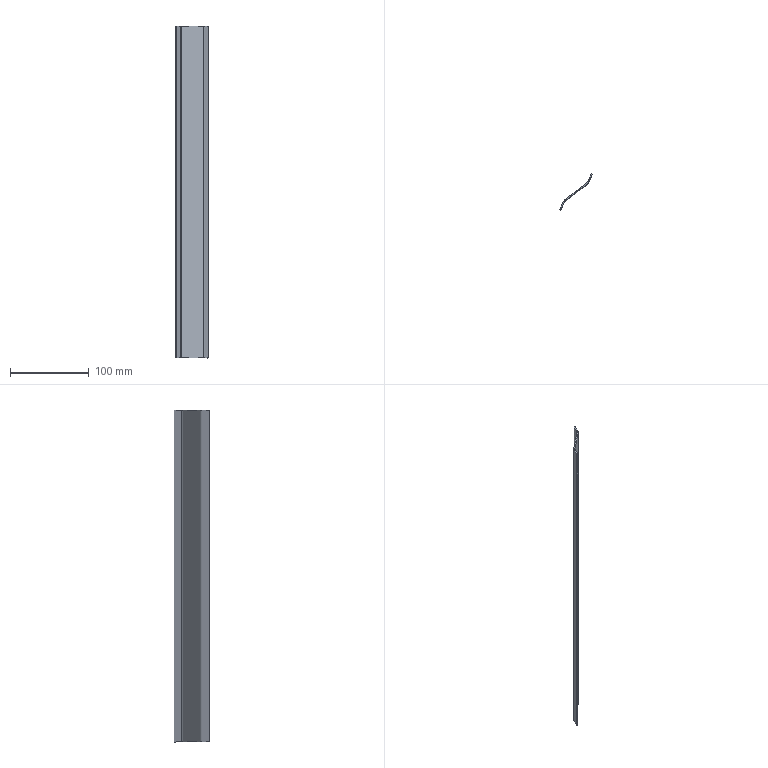Part | STEP file | 750038406 | 1 solid | 14 faces | box 41.359 x 45.634 x 422 mm | volume 39080 mm3 | plane 10 | cylinder 4 | commonest cylinder face diameters 10 x2 13 x2
STEP:
#1=CARTESIAN_POINT('',(6.307,11.838,211.));
#2=VERTEX_POINT('',#1);
#3=CARTESIAN_POINT('',(33.978,33.384,211.));
#4=VERTEX_POINT('',#3);
#5=CARTESIAN_POINT('',(5.071,10.876,211.));
#6=DIRECTION('',(0.789,0.6144,0.));
#7=VECTOR('',#6,1000.);
#8=LINE('',#5,#7);
#9=EDGE_CURVE('',#2,#4,#8,.T.);
#10=ORIENTED_EDGE('',*,*,#9,.T.);
#11=CARTESIAN_POINT('',(33.978,33.384,-211.));
#12=VERTEX_POINT('',#11);
#13=CARTESIAN_POINT('',(33.978,33.384,211.));
#14=DIRECTION('',(0.,0.,-1.));
#15=VECTOR('',#14,1000.);
#16=LINE('',#13,#15);
#17=EDGE_CURVE('',#4,#12,#16,.T.);
#18=ORIENTED_EDGE('',*,*,#17,.T.);
#19=CARTESIAN_POINT('',(6.307,11.838,-211.));
#20=VERTEX_POINT('',#19);
#21=CARTESIAN_POINT('',(5.071,10.876,-211.));
#22=DIRECTION('',(-0.789,-0.6144,0.));
#23=VECTOR('',#22,1000.);
#24=LINE('',#21,#23);
#25=EDGE_CURVE('',#12,#20,#24,.T.);
#26=ORIENTED_EDGE('',*,*,#25,.T.);
#27=CARTESIAN_POINT('',(6.307,11.838,211.));
#28=DIRECTION('',(0.,0.,1.));
#29=VECTOR('',#28,1000.);
#30=LINE('',#27,#29);
#31=EDGE_CURVE('',#20,#2,#30,.T.);
#32=ORIENTED_EDGE('',*,*,#31,.T.);
#33=EDGE_LOOP('',(#10,#18,#26,#32));
#34=FACE_OUTER_BOUND('',#33,.T.);
#35=CARTESIAN_POINT('',(5.071,10.876,211.));
#36=DIRECTION('',(-0.6144,0.789,0.));
#37=DIRECTION('',(-0.789,-0.6144,0.));
#38=AXIS2_PLACEMENT_3D('',#35,#36,#37);
#39=PLANE('',#38);
#40=ADVANCED_FACE('',(#34),#39,.T.);
#41=ORIENTED_EDGE('',*,*,#17,.F.);
#42=CARTESIAN_POINT('',(35.438,35.216,211.));
#43=VERTEX_POINT('',#42);
#44=CARTESIAN_POINT('',(30.906,37.329,211.));
#45=DIRECTION('',(0.,0.,-1.));
#46=DIRECTION('',(-1.,0.,0.));
#47=AXIS2_PLACEMENT_3D('',#44,#45,#46);
#48=CIRCLE('',#47,5.);
#49=EDGE_CURVE('',#43,#4,#48,.T.);
#50=ORIENTED_EDGE('',*,*,#49,.F.);
#51=CARTESIAN_POINT('',(35.438,35.216,-211.));
#52=VERTEX_POINT('',#51);
#53=CARTESIAN_POINT('',(35.438,35.216,211.));
#54=DIRECTION('',(0.,0.,1.));
#55=VECTOR('',#54,1000.);
#56=LINE('',#53,#55);
#57=EDGE_CURVE('',#52,#43,#56,.T.);
#58=ORIENTED_EDGE('',*,*,#57,.F.);
#59=CARTESIAN_POINT('',(30.906,37.329,-211.));
#60=DIRECTION('',(0.,0.,1.));
#61=DIRECTION('',(-1.,0.,0.));
#62=AXIS2_PLACEMENT_3D('',#59,#60,#61);
#63=CIRCLE('',#62,5.);
#64=EDGE_CURVE('',#12,#52,#63,.T.);
#65=ORIENTED_EDGE('',*,*,#64,.F.);
#66=EDGE_LOOP('',(#41,#50,#58,#65));
#67=FACE_OUTER_BOUND('',#66,.T.);
#68=CARTESIAN_POINT('',(30.906,37.329,211.));
#69=DIRECTION('',(0.,0.,-1.));
#70=DIRECTION('',(-1.,0.,0.));
#71=AXIS2_PLACEMENT_3D('',#68,#69,#70);
#72=CYLINDRICAL_SURFACE('',#71,5.);
#73=ADVANCED_FACE('',(#67),#72,.F.);
#74=CARTESIAN_POINT('',(36.797,34.582,211.));
#75=VERTEX_POINT('',#74);
#76=CARTESIAN_POINT('',(41.359,44.366,211.));
#77=VERTEX_POINT('',#76);
#78=CARTESIAN_POINT('',(36.797,34.582,211.));
#79=DIRECTION('',(0.4226,0.9063,0.));
#80=VECTOR('',#79,1000.);
#81=LINE('',#78,#80);
#82=EDGE_CURVE('',#75,#77,#81,.T.);
#83=ORIENTED_EDGE('',*,*,#82,.T.);
#84=CARTESIAN_POINT('',(40.,45.,211.));
#85=VERTEX_POINT('',#84);
#86=CARTESIAN_POINT('',(40.,45.,211.));
#87=DIRECTION('',(0.9063,-0.4226,0.));
#88=VECTOR('',#87,1000.);
#89=LINE('',#86,#88);
#90=EDGE_CURVE('',#85,#77,#89,.T.);
#91=ORIENTED_EDGE('',*,*,#90,.F.);
#92=CARTESIAN_POINT('',(40.,45.,211.));
#93=DIRECTION('',(-0.4226,-0.9063,0.));
#94=VECTOR('',#93,1000.);
#95=LINE('',#92,#94);
#96=EDGE_CURVE('',#85,#43,#95,.T.);
#97=ORIENTED_EDGE('',*,*,#96,.T.);
#98=ORIENTED_EDGE('',*,*,#49,.T.);
#99=ORIENTED_EDGE('',*,*,#9,.F.);
#100=CARTESIAN_POINT('',(4.41,9.456,211.));
#101=VERTEX_POINT('',#100);
#102=CARTESIAN_POINT('',(10.301,6.709,211.));
#103=DIRECTION('',(0.,0.,1.));
#104=DIRECTION('',(-1.,0.,0.));
#105=AXIS2_PLACEMENT_3D('',#102,#103,#104);
#106=CIRCLE('',#105,6.5);
#107=EDGE_CURVE('',#2,#101,#106,.T.);
#108=ORIENTED_EDGE('',*,*,#107,.T.);
#109=CARTESIAN_POINT('',(0.,0.,211.));
#110=VERTEX_POINT('',#109);
#111=CARTESIAN_POINT('',(4.41,9.456,211.));
#112=DIRECTION('',(-0.4226,-0.9063,0.));
#113=VECTOR('',#112,1000.);
#114=LINE('',#111,#113);
#115=EDGE_CURVE('',#101,#110,#114,.T.);
#116=ORIENTED_EDGE('',*,*,#115,.T.);
#117=CARTESIAN_POINT('',(1.359,-0.6339,211.));
#118=VERTEX_POINT('',#117);
#119=CARTESIAN_POINT('',(0.,0.,211.));
#120=DIRECTION('',(0.9063,-0.4226,0.));
#121=VECTOR('',#120,1000.);
#122=LINE('',#119,#121);
#123=EDGE_CURVE('',#110,#118,#122,.T.);
#124=ORIENTED_EDGE('',*,*,#123,.T.);
#125=CARTESIAN_POINT('',(5.769,8.822,211.));
#126=VERTEX_POINT('',#125);
#127=CARTESIAN_POINT('',(1.359,-0.6339,211.));
#128=DIRECTION('',(0.4226,0.9063,0.));
#129=VECTOR('',#128,1000.);
#130=LINE('',#127,#129);
#131=EDGE_CURVE('',#118,#126,#130,.T.);
#132=ORIENTED_EDGE('',*,*,#131,.T.);
#133=CARTESIAN_POINT('',(7.229,10.654,211.));
#134=VERTEX_POINT('',#133);
#135=CARTESIAN_POINT('',(10.301,6.709,211.));
#136=DIRECTION('',(0.,0.,-1.));
#137=DIRECTION('',(-1.,0.,0.));
#138=AXIS2_PLACEMENT_3D('',#135,#136,#137);
#139=CIRCLE('',#138,5.);
#140=EDGE_CURVE('',#126,#134,#139,.T.);
#141=ORIENTED_EDGE('',*,*,#140,.T.);
#142=CARTESIAN_POINT('',(34.9,32.201,211.));
#143=VERTEX_POINT('',#142);
#144=CARTESIAN_POINT('',(7.229,10.654,211.));
#145=DIRECTION('',(0.789,0.6144,0.));
#146=VECTOR('',#145,1000.);
#147=LINE('',#144,#146);
#148=EDGE_CURVE('',#134,#143,#147,.T.);
#149=ORIENTED_EDGE('',*,*,#148,.T.);
#150=CARTESIAN_POINT('',(30.906,37.329,211.));
#151=DIRECTION('',(0.,0.,1.));
#152=DIRECTION('',(-1.,0.,0.));
#153=AXIS2_PLACEMENT_3D('',#150,#151,#152);
#154=CIRCLE('',#153,6.5);
#155=EDGE_CURVE('',#143,#75,#154,.T.);
#156=ORIENTED_EDGE('',*,*,#155,.T.);
#157=EDGE_LOOP('',(#83,#91,#97,#98,#99,#108,#116,#124,#132,#141,#149,#156));
#158=FACE_OUTER_BOUND('',#157,.T.);
#159=CARTESIAN_POINT('',(34.929,34.124,211.));
#160=DIRECTION('',(0.,0.,1.));
#161=DIRECTION('',(1.,0.,0.));
#162=AXIS2_PLACEMENT_3D('',#159,#160,#161);
#163=PLANE('',#162);
#164=ADVANCED_FACE('',(#158),#163,.T.);
#165=ORIENTED_EDGE('',*,*,#107,.F.);
#166=ORIENTED_EDGE('',*,*,#31,.F.);
#167=CARTESIAN_POINT('',(4.41,9.456,-211.));
#168=VERTEX_POINT('',#167);
#169=CARTESIAN_POINT('',(10.301,6.709,-211.));
#170=DIRECTION('',(0.,0.,1.));
#171=DIRECTION('',(-1.,0.,0.));
#172=AXIS2_PLACEMENT_3D('',#169,#170,#171);
#173=CIRCLE('',#172,6.5);
#174=EDGE_CURVE('',#20,#168,#173,.T.);
#175=ORIENTED_EDGE('',*,*,#174,.T.);
#176=CARTESIAN_POINT('',(4.41,9.456,211.));
#177=DIRECTION('',(0.,0.,1.));
#178=VECTOR('',#177,1000.);
#179=LINE('',#176,#178);
#180=EDGE_CURVE('',#168,#101,#179,.T.);
#181=ORIENTED_EDGE('',*,*,#180,.T.);
#182=EDGE_LOOP('',(#165,#166,#175,#181));
#183=FACE_OUTER_BOUND('',#182,.T.);
#184=CARTESIAN_POINT('',(10.301,6.709,211.));
#185=DIRECTION('',(0.,0.,-1.));
#186=DIRECTION('',(-1.,0.,0.));
#187=AXIS2_PLACEMENT_3D('',#184,#185,#186);
#188=CYLINDRICAL_SURFACE('',#187,6.5);
#189=ADVANCED_FACE('',(#183),#188,.T.);
#190=ORIENTED_EDGE('',*,*,#174,.F.);
#191=ORIENTED_EDGE('',*,*,#25,.F.);
#192=ORIENTED_EDGE('',*,*,#64,.T.);
#193=CARTESIAN_POINT('',(40.,45.,-211.));
#194=VERTEX_POINT('',#193);
#195=CARTESIAN_POINT('',(40.,45.,-211.));
#196=DIRECTION('',(-0.4226,-0.9063,0.));
#197=VECTOR('',#196,1000.);
#198=LINE('',#195,#197);
#199=EDGE_CURVE('',#194,#52,#198,.T.);
#200=ORIENTED_EDGE('',*,*,#199,.F.);
#201=CARTESIAN_POINT('',(41.359,44.366,-211.));
#202=VERTEX_POINT('',#201);
#203=CARTESIAN_POINT('',(40.,45.,-211.));
#204=DIRECTION('',(-0.9063,0.4226,0.));
#205=VECTOR('',#204,1000.);
#206=LINE('',#203,#205);
#207=EDGE_CURVE('',#202,#194,#206,.T.);
#208=ORIENTED_EDGE('',*,*,#207,.F.);
#209=CARTESIAN_POINT('',(36.797,34.582,-211.));
#210=VERTEX_POINT('',#209);
#211=CARTESIAN_POINT('',(36.797,34.582,-211.));
#212=DIRECTION('',(0.4226,0.9063,0.));
#213=VECTOR('',#212,1000.);
#214=LINE('',#211,#213);
#215=EDGE_CURVE('',#210,#202,#214,.T.);
#216=ORIENTED_EDGE('',*,*,#215,.F.);
#217=CARTESIAN_POINT('',(34.9,32.201,-211.));
#218=VERTEX_POINT('',#217);
#219=CARTESIAN_POINT('',(30.906,37.329,-211.));
#220=DIRECTION('',(0.,0.,1.));
#221=DIRECTION('',(-1.,0.,0.));
#222=AXIS2_PLACEMENT_3D('',#219,#220,#221);
#223=CIRCLE('',#222,6.5);
#224=EDGE_CURVE('',#218,#210,#223,.T.);
#225=ORIENTED_EDGE('',*,*,#224,.F.);
#226=CARTESIAN_POINT('',(7.229,10.654,-211.));
#227=VERTEX_POINT('',#226);
#228=CARTESIAN_POINT('',(7.229,10.654,-211.));
#229=DIRECTION('',(0.789,0.6144,0.));
#230=VECTOR('',#229,1000.);
#231=LINE('',#228,#230);
#232=EDGE_CURVE('',#227,#218,#231,.T.);
#233=ORIENTED_EDGE('',*,*,#232,.F.);
#234=CARTESIAN_POINT('',(5.769,8.822,-211.));
#235=VERTEX_POINT('',#234);
#236=CARTESIAN_POINT('',(10.301,6.709,-211.));
#237=DIRECTION('',(0.,0.,-1.));
#238=DIRECTION('',(-1.,0.,0.));
#239=AXIS2_PLACEMENT_3D('',#236,#237,#238);
#240=CIRCLE('',#239,5.);
#241=EDGE_CURVE('',#235,#227,#240,.T.);
#242=ORIENTED_EDGE('',*,*,#241,.F.);
#243=CARTESIAN_POINT('',(1.359,-0.6339,-211.));
#244=VERTEX_POINT('',#243);
#245=CARTESIAN_POINT('',(1.359,-0.6339,-211.));
#246=DIRECTION('',(0.4226,0.9063,0.));
#247=VECTOR('',#246,1000.);
#248=LINE('',#245,#247);
#249=EDGE_CURVE('',#244,#235,#248,.T.);
#250=ORIENTED_EDGE('',*,*,#249,.F.);
#251=CARTESIAN_POINT('',(0.,0.,-211.));
#252=VERTEX_POINT('',#251);
#253=CARTESIAN_POINT('',(0.,0.,-211.));
#254=DIRECTION('',(-0.9063,0.4226,0.));
#255=VECTOR('',#254,1000.);
#256=LINE('',#253,#255);
#257=EDGE_CURVE('',#244,#252,#256,.T.);
#258=ORIENTED_EDGE('',*,*,#257,.T.);
#259=CARTESIAN_POINT('',(4.41,9.456,-211.));
#260=DIRECTION('',(-0.4226,-0.9063,0.));
#261=VECTOR('',#260,1000.);
#262=LINE('',#259,#261);
#263=EDGE_CURVE('',#168,#252,#262,.T.);
#264=ORIENTED_EDGE('',*,*,#263,.F.);
#265=EDGE_LOOP('',(#190,#191,#192,#200,#208,#216,#225,#233,#242,#250,#258,#264));
#266=FACE_OUTER_BOUND('',#265,.T.);
#267=CARTESIAN_POINT('',(0.,0.,-211.));
#268=DIRECTION('',(0.,0.,1.));
#269=DIRECTION('',(1.,0.,0.));
#270=AXIS2_PLACEMENT_3D('',#267,#268,#269);
#271=PLANE('',#270);
#272=ADVANCED_FACE('',(#266),#271,.F.);
#273=ORIENTED_EDGE('',*,*,#96,.F.);
#274=CARTESIAN_POINT('',(40.,45.,211.));
#275=DIRECTION('',(0.,0.,-1.));
#276=VECTOR('',#275,1000.);
#277=LINE('',#274,#276);
#278=EDGE_CURVE('',#85,#194,#277,.T.);
#279=ORIENTED_EDGE('',*,*,#278,.T.);
#280=ORIENTED_EDGE('',*,*,#199,.T.);
#281=ORIENTED_EDGE('',*,*,#57,.T.);
#282=EDGE_LOOP('',(#273,#279,#280,#281));
#283=FACE_OUTER_BOUND('',#282,.T.);
#284=CARTESIAN_POINT('',(34.929,34.124,211.));
#285=DIRECTION('',(-0.9063,0.4226,0.));
#286=DIRECTION('',(-0.4226,-0.9063,0.));
#287=AXIS2_PLACEMENT_3D('',#284,#285,#286);
#288=PLANE('',#287);
#289=ADVANCED_FACE('',(#283),#288,.T.);
#290=CARTESIAN_POINT('',(41.359,44.366,211.));
#291=DIRECTION('',(0.,0.,-1.));
#292=VECTOR('',#291,1000.);
#293=LINE('',#290,#292);
#294=EDGE_CURVE('',#77,#202,#293,.T.);
#295=ORIENTED_EDGE('',*,*,#294,.F.);
#296=ORIENTED_EDGE('',*,*,#82,.F.);
#297=CARTESIAN_POINT('',(36.797,34.582,211.));
#298=DIRECTION('',(0.,0.,1.));
#299=VECTOR('',#298,1000.);
#300=LINE('',#297,#299);
#301=EDGE_CURVE('',#210,#75,#300,.T.);
#302=ORIENTED_EDGE('',*,*,#301,.F.);
#303=ORIENTED_EDGE('',*,*,#215,.T.);
#304=EDGE_LOOP('',(#295,#296,#302,#303));
#305=FACE_OUTER_BOUND('',#304,.T.);
#306=CARTESIAN_POINT('',(36.288,33.49,211.));
#307=DIRECTION('',(-0.9063,0.4226,0.));
#308=DIRECTION('',(-0.4226,-0.9063,0.));
#309=AXIS2_PLACEMENT_3D('',#306,#307,#308);
#310=PLANE('',#309);
#311=ADVANCED_FACE('',(#305),#310,.F.);
#312=ORIENTED_EDGE('',*,*,#155,.F.);
#313=CARTESIAN_POINT('',(34.9,32.201,211.));
#314=DIRECTION('',(0.,0.,-1.));
#315=VECTOR('',#314,1000.);
#316=LINE('',#313,#315);
#317=EDGE_CURVE('',#143,#218,#316,.T.);
#318=ORIENTED_EDGE('',*,*,#317,.T.);
#319=ORIENTED_EDGE('',*,*,#224,.T.);
#320=ORIENTED_EDGE('',*,*,#301,.T.);
#321=EDGE_LOOP('',(#312,#318,#319,#320));
#322=FACE_OUTER_BOUND('',#321,.T.);
#323=CARTESIAN_POINT('',(30.906,37.329,211.));
#324=DIRECTION('',(0.,0.,-1.));
#325=DIRECTION('',(-1.,0.,0.));
#326=AXIS2_PLACEMENT_3D('',#323,#324,#325);
#327=CYLINDRICAL_SURFACE('',#326,6.5);
#328=ADVANCED_FACE('',(#322),#327,.T.);
#329=ORIENTED_EDGE('',*,*,#317,.F.);
#330=ORIENTED_EDGE('',*,*,#148,.F.);
#331=CARTESIAN_POINT('',(7.229,10.654,211.));
#332=DIRECTION('',(0.,0.,1.));
#333=VECTOR('',#332,1000.);
#334=LINE('',#331,#333);
#335=EDGE_CURVE('',#227,#134,#334,.T.);
#336=ORIENTED_EDGE('',*,*,#335,.F.);
#337=ORIENTED_EDGE('',*,*,#232,.T.);
#338=EDGE_LOOP('',(#329,#330,#336,#337));
#339=FACE_OUTER_BOUND('',#338,.T.);
#340=CARTESIAN_POINT('',(5.993,9.692,211.));
#341=DIRECTION('',(-0.6144,0.789,0.));
#342=DIRECTION('',(-0.789,-0.6144,0.));
#343=AXIS2_PLACEMENT_3D('',#340,#341,#342);
#344=PLANE('',#343);
#345=ADVANCED_FACE('',(#339),#344,.F.);
#346=ORIENTED_EDGE('',*,*,#335,.T.);
#347=ORIENTED_EDGE('',*,*,#140,.F.);
#348=CARTESIAN_POINT('',(5.769,8.822,211.));
#349=DIRECTION('',(0.,0.,1.));
#350=VECTOR('',#349,1000.);
#351=LINE('',#348,#350);
#352=EDGE_CURVE('',#235,#126,#351,.T.);
#353=ORIENTED_EDGE('',*,*,#352,.F.);
#354=ORIENTED_EDGE('',*,*,#241,.T.);
#355=EDGE_LOOP('',(#346,#347,#353,#354));
#356=FACE_OUTER_BOUND('',#355,.T.);
#357=CARTESIAN_POINT('',(10.301,6.709,211.));
#358=DIRECTION('',(0.,0.,-1.));
#359=DIRECTION('',(-1.,0.,0.));
#360=AXIS2_PLACEMENT_3D('',#357,#358,#359);
#361=CYLINDRICAL_SURFACE('',#360,5.);
#362=ADVANCED_FACE('',(#356),#361,.F.);
#363=ORIENTED_EDGE('',*,*,#352,.T.);
#364=ORIENTED_EDGE('',*,*,#131,.F.);
#365=CARTESIAN_POINT('',(1.359,-0.6339,211.));
#366=DIRECTION('',(0.,0.,1.));
#367=VECTOR('',#366,1000.);
#368=LINE('',#365,#367);
#369=EDGE_CURVE('',#244,#118,#368,.T.);
#370=ORIENTED_EDGE('',*,*,#369,.F.);
#371=ORIENTED_EDGE('',*,*,#249,.T.);
#372=EDGE_LOOP('',(#363,#364,#370,#371));
#373=FACE_OUTER_BOUND('',#372,.T.);
#374=CARTESIAN_POINT('',(1.359,-0.6339,211.));
#375=DIRECTION('',(-0.9063,0.4226,0.));
#376=DIRECTION('',(-0.4226,-0.9063,0.));
#377=AXIS2_PLACEMENT_3D('',#374,#375,#376);
#378=PLANE('',#377);
#379=ADVANCED_FACE('',(#373),#378,.F.);
#380=ORIENTED_EDGE('',*,*,#115,.F.);
#381=ORIENTED_EDGE('',*,*,#180,.F.);
#382=ORIENTED_EDGE('',*,*,#263,.T.);
#383=CARTESIAN_POINT('',(0.,0.,211.));
#384=DIRECTION('',(0.,0.,1.));
#385=VECTOR('',#384,1000.);
#386=LINE('',#383,#385);
#387=EDGE_CURVE('',#252,#110,#386,.T.);
#388=ORIENTED_EDGE('',*,*,#387,.T.);
#389=EDGE_LOOP('',(#380,#381,#382,#388));
#390=FACE_OUTER_BOUND('',#389,.T.);
#391=CARTESIAN_POINT('',(0.,0.,211.));
#392=DIRECTION('',(-0.9063,0.4226,0.));
#393=DIRECTION('',(-0.4226,-0.9063,0.));
#394=AXIS2_PLACEMENT_3D('',#391,#392,#393);
#395=PLANE('',#394);
#396=ADVANCED_FACE('',(#390),#395,.T.);
#397=ORIENTED_EDGE('',*,*,#207,.T.);
#398=ORIENTED_EDGE('',*,*,#278,.F.);
#399=ORIENTED_EDGE('',*,*,#90,.T.);
#400=ORIENTED_EDGE('',*,*,#294,.T.);
#401=EDGE_LOOP('',(#397,#398,#399,#400));
#402=FACE_OUTER_BOUND('',#401,.T.);
#403=CARTESIAN_POINT('',(40.,45.,211.));
#404=DIRECTION('',(0.4226,0.9063,0.));
#405=DIRECTION('',(-0.9063,0.4226,0.));
#406=AXIS2_PLACEMENT_3D('',#403,#404,#405);
#407=PLANE('',#406);
#408=ADVANCED_FACE('',(#402),#407,.T.);
#409=ORIENTED_EDGE('',*,*,#123,.F.);
#410=ORIENTED_EDGE('',*,*,#387,.F.);
#411=ORIENTED_EDGE('',*,*,#257,.F.);
#412=ORIENTED_EDGE('',*,*,#369,.T.);
#413=EDGE_LOOP('',(#409,#410,#411,#412));
#414=FACE_OUTER_BOUND('',#413,.T.);
#415=CARTESIAN_POINT('',(0.,0.,211.));
#416=DIRECTION('',(0.4226,0.9063,0.));
#417=DIRECTION('',(-0.9063,0.4226,0.));
#418=AXIS2_PLACEMENT_3D('',#415,#416,#417);
#419=PLANE('',#418);
#420=ADVANCED_FACE('',(#414),#419,.F.);
#421=CLOSED_SHELL('',(#40,#73,#164,#189,#272,#289,#311,#328,#345,#362,#379,#396,#408,#420));
#422=MANIFOLD_SOLID_BREP('',#421);
#423=CARTESIAN_POINT('',(0.,0.,0.));
#424=DIRECTION('',(0.,0.,1.));
#425=DIRECTION('',(1.,0.,0.));
#426=AXIS2_PLACEMENT_3D('',#423,#424,#425);
#427=(LENGTH_UNIT()NAMED_UNIT(*)SI_UNIT(.MILLI.,.METRE.));
#428=UNCERTAINTY_MEASURE_WITH_UNIT(LENGTH_MEASURE(0.00001),#427,'','');
#429=(NAMED_UNIT(*)PLANE_ANGLE_UNIT()SI_UNIT($,.RADIAN.));
#430=(NAMED_UNIT(*)SI_UNIT($,.STERADIAN.)SOLID_ANGLE_UNIT());
#431=(GEOMETRIC_REPRESENTATION_CONTEXT(3)GLOBAL_UNCERTAINTY_ASSIGNED_CONTEXT((#428))GLOBAL_UNIT_ASSIGNED_CONTEXT((#427,#429,#430))REPRESENTATION_CONTEXT('',''));
#432=ADVANCED_BREP_SHAPE_REPRESENTATION('',(#422,#426),#431);